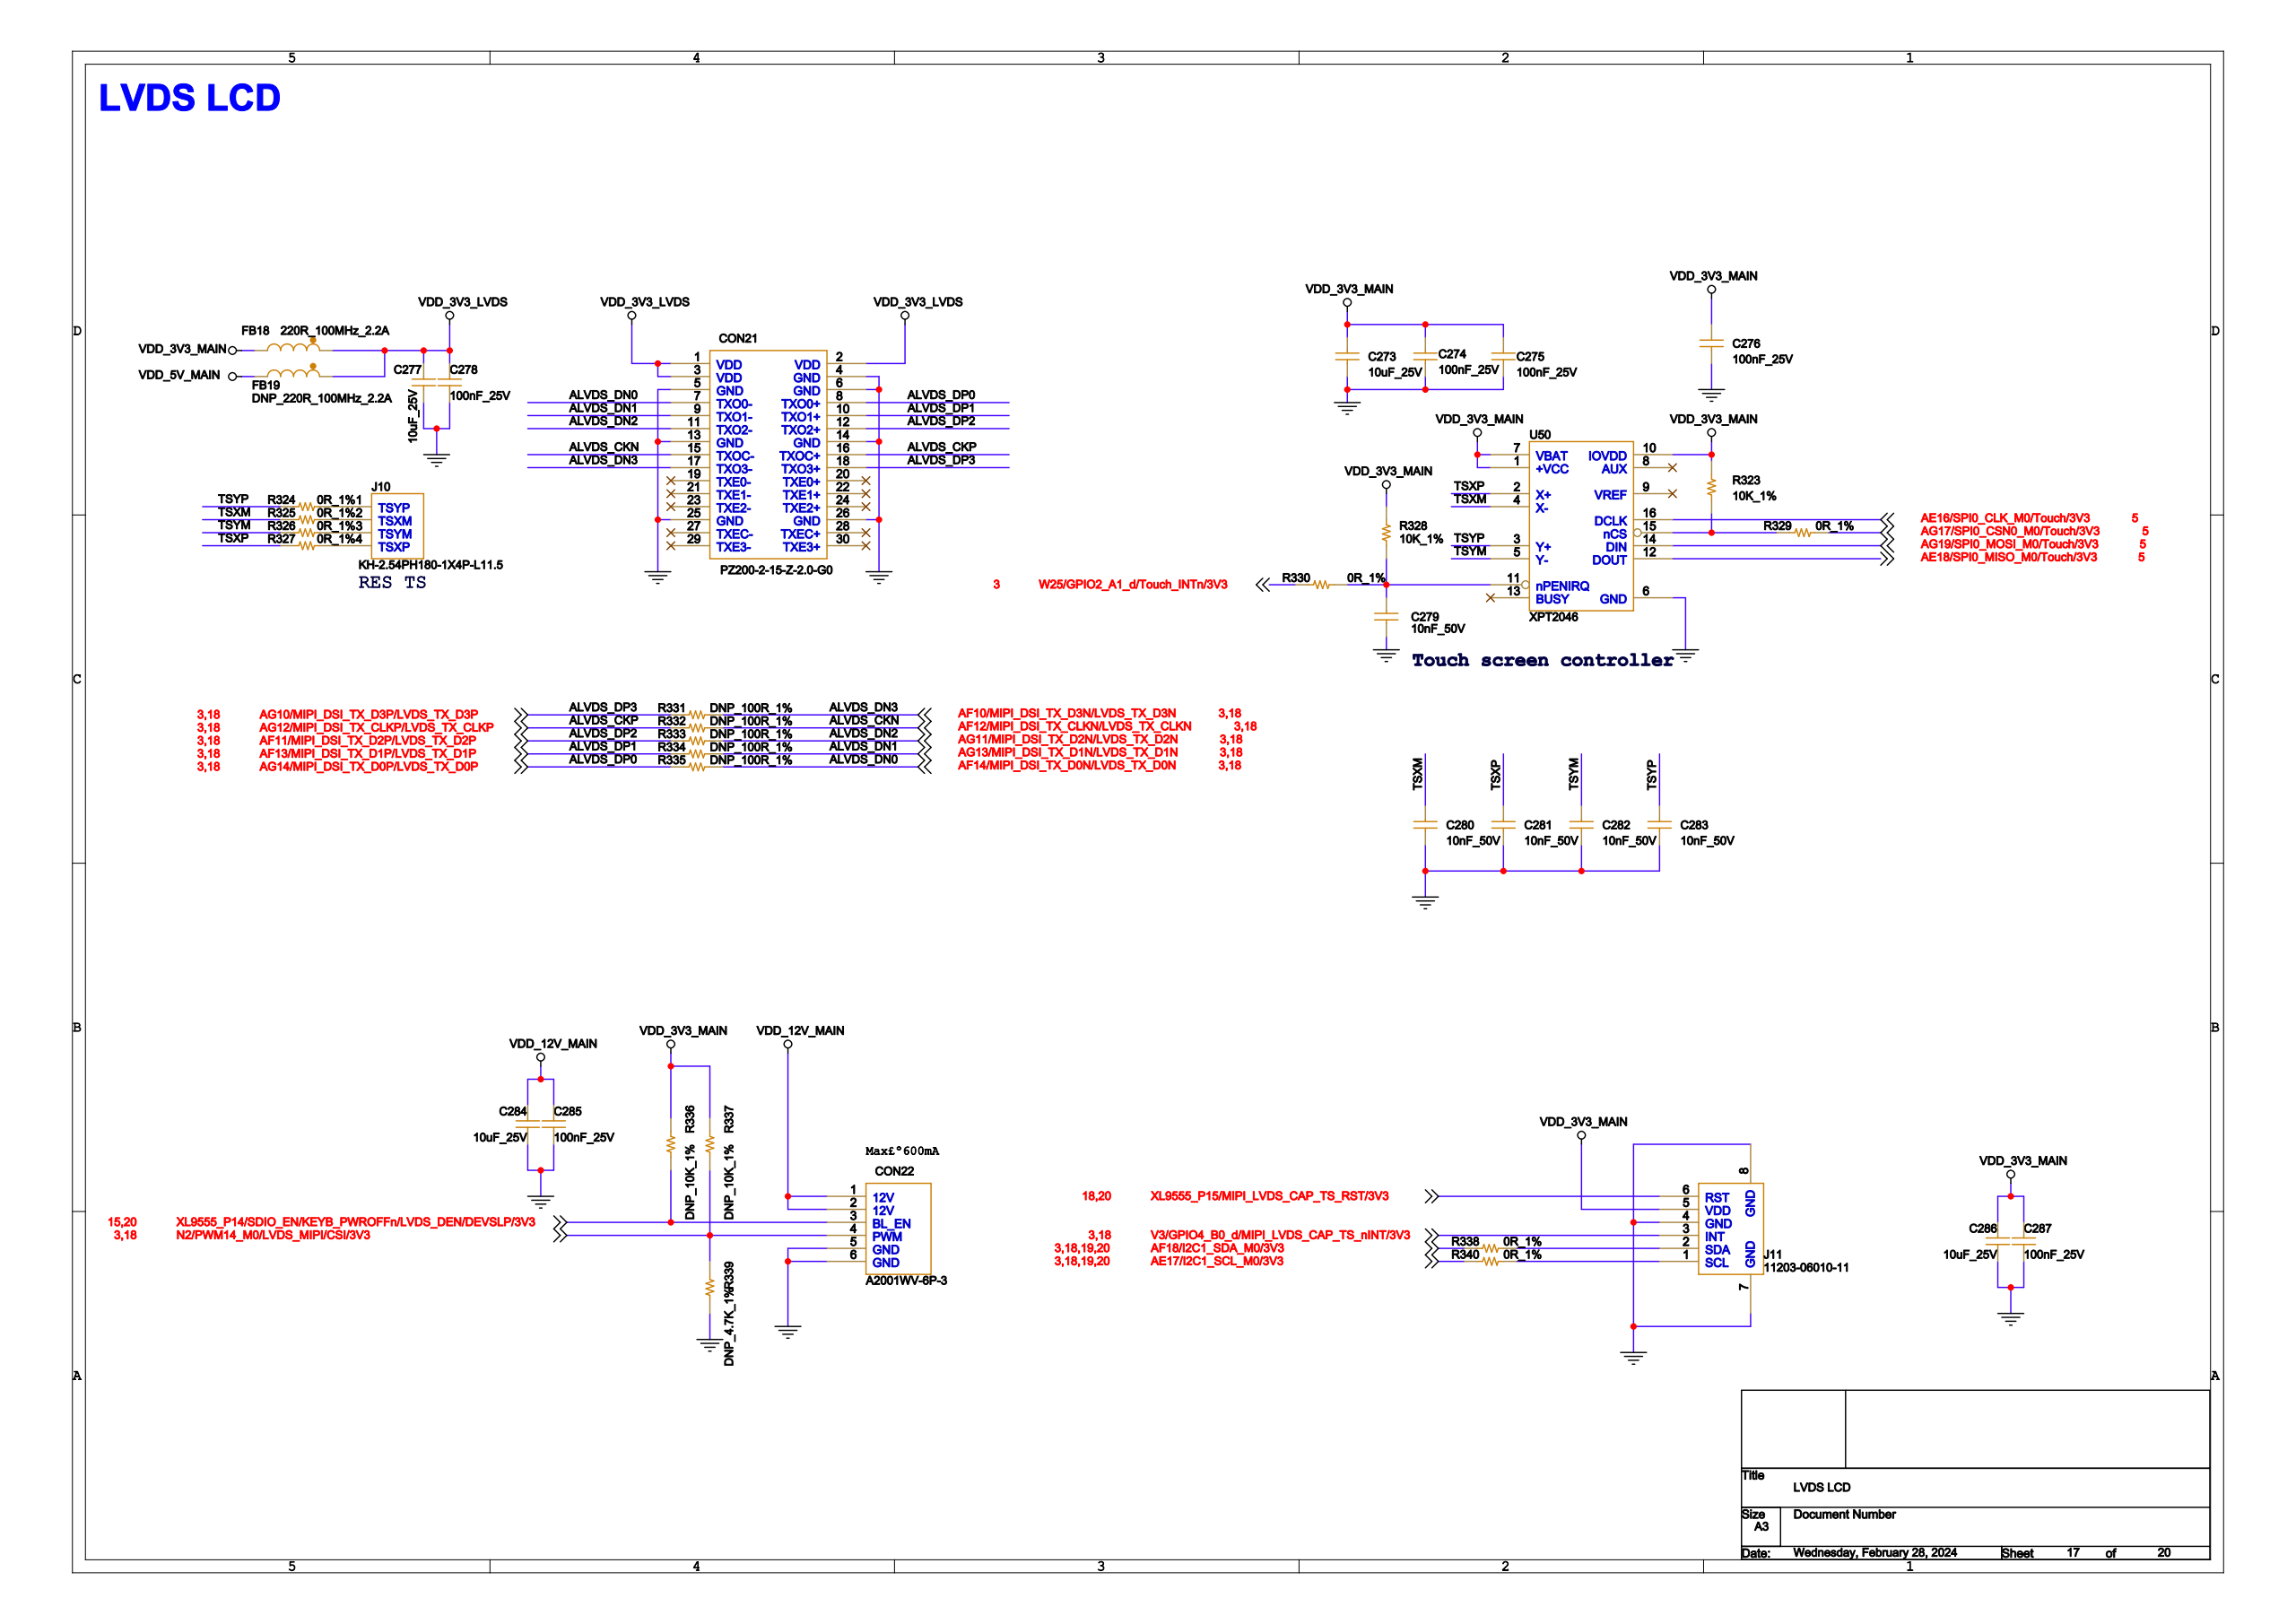Circuit board | Cadence Allegro | 1024 parts | 682 nets | one sheet of the schematic
Parts on this sheet (reference | value | footprint):
C273 | 10uF_25V | C0603
C274 | 100nF_25V | C0402
C275 | 100nF_25V | C0402
C276 | 100nF_25V | C0402
C278 | 100nF_25V | C0402
C279 | 10nF_50V | C0402
C280 | 10nF_50V | C0402
C281 | 10nF_50V | C0402
C282 | 10nF_50V | C0402
C283 | 10nF_50V | C0402
C284 | 10uF_25V | C0603
C285 | 100nF_25V | C0402
C286 | 10uF_25V | C0603
C287 | 100nF_25V | C0402
CON21 | PZ200-2-15-Z-2.0-G0 | CON_2MM_2X15P
CON22 | A2001WV-6P-3 | CON_PHD_2D0_1X6P_TH_180
FB18 | 220R_100MHz_2A | L0603
FB19 | DNP_220R_100MHz_2A | L0603
J10 | KH-2.54PH180-1X4P-L11.5 | CON_TH_1X4P_2D54_H_DIP
J11 | 11203-06010-11 | CON_FFC_0D5_6P
R323 | 10K_1% | R0402
R324 | 0R_1% | R0402
R325 | 0R_1% | R0402
R326 | 0R_1% | R0402
R327 | 0R_1% | R0402
R328 | 10K_1% | R0402
R329 | 0R_1% | R0402
R330 | 0R_1% | R0402
R331 | DNP_100R_1% | R0402
R332 | DNP_100R_1% | R0402
R333 | DNP_100R_1% | R0402
R334 | DNP_100R_1% | R0402
R335 | DNP_100R_1% | R0402
R336 | DNP_10K_1% | R0402
R337 | DNP_10K_1% | R0402
R338 | 0R_1% | R0402
R339 | DNP_4.7K_1% | R0402
R340 | 0R_1% | R0402
U50 | XPT2046 | TSSOP16_PW16
Nets of these parts (net: part-pin ...):
GND: C273-2 C274-2 C275-2 C276-2 C278-2 C279-2 C280-2 C281-2 C282-2 C283-2 C284-2 C285-2 C286-2 C287-2 CON21-4 CON21-5 CON21-6 CON21-13 CON21-14 CON21-25 CON21-26 CON22-5 CON22-6 J11-4 J11-7 J11-8 R339-2 U50-6
VDD_5V_MAIN: FB19-2
AF10/MIPI_DSI_TX_D3N/LVDS_TX_D3: CON21-17 R331-1
AG10/MIPI_DSI_TX_D3P/LVDS_TX_D3: CON21-18 R331-2
AF12/MIPI_DSI_TX_CLKN/LVDS_TX_C: CON21-15 R332-1
AG12/MIPI_DSI_TX_CLKP/LVDS_TX_C: CON21-16 R332-2
AG11/MIPI_DSI_TX_D2N/LVDS_TX_D2: CON21-11 R333-1
AF11/MIPI_DSI_TX_D2P/LVDS_TX_D2: CON21-12 R333-2
AG13/MIPI_DSI_TX_D1N/LVDS_TX_D1: CON21-9 R334-1
AF13/MIPI_DSI_TX_D1P/LVDS_TX_D1: CON21-10 R334-2
AF14/MIPI_DSI_TX_D0N/LVDS_TX_D0: CON21-7 R335-1
AG14/MIPI_DSI_TX_D0P/LVDS_TX_D0: CON21-8 R335-2
VDD_3V3_LVDS: C278-1 CON21-1 CON21-2 CON21-3 FB18-1 FB19-1
VDD_3V3_MAIN: C273-1 C274-1 C275-1 C276-1 C286-1 C287-1 FB18-2 J11-5 R323-1 R328-1 R336-1 R337-1 U50-1 U50-7 U50-10
N21716785: C279-1 R328-2 R330-2 U50-11
TSXM: C280-1 R325-2 U50-4
TSXP: C281-1 R327-2 U50-2
TSYM: C282-1 R326-2 U50-5
TSYP: C283-1 R324-2 U50-3
W25/GPIO2_A1_D/TOUCH_INTN/3V3: R330-1
AF18/I2C1_SDA_M0/3V3: R338-1
AE17/I2C1_SCL_M0/3V3: R340-1
V3/GPIO4_B0_D/MIPI_LVDS_CAP_TS_: J11-3
N2/PWM14_M0/LVDS_MIPI/CSI/3V3: CON22-4 R337-2 R339-1
N217147881: J10-2 R325-1
N217147883: J10-4 R327-1
N217147882: J10-3 R326-1
N217147880: J10-1 R324-1
XL9555_P15/MIPI_LVDS_CAP_TS_RST: J11-6
N21719855: J11-1 R340-2
N21719858: J11-2 R338-2
VDD_12V_MAIN: C284-1 C285-1 CON22-1 CON22-2
XL9555_P14/SDIO_EN/KEYB_PWROFFN: CON22-3 R336-2
N21716697: R323-2 R329-1 U50-15
AG17/SPI0_CSN0_M0/TOUCH/3V3: R329-2
AG19/SPI0_MOSI_M0/TOUCH/3V3: U50-14
AE18/SPI0_MISO_M0/TOUCH/3V3: U50-12
AE16/SPI0_CLK_M0/TOUCH/3V3: U50-16